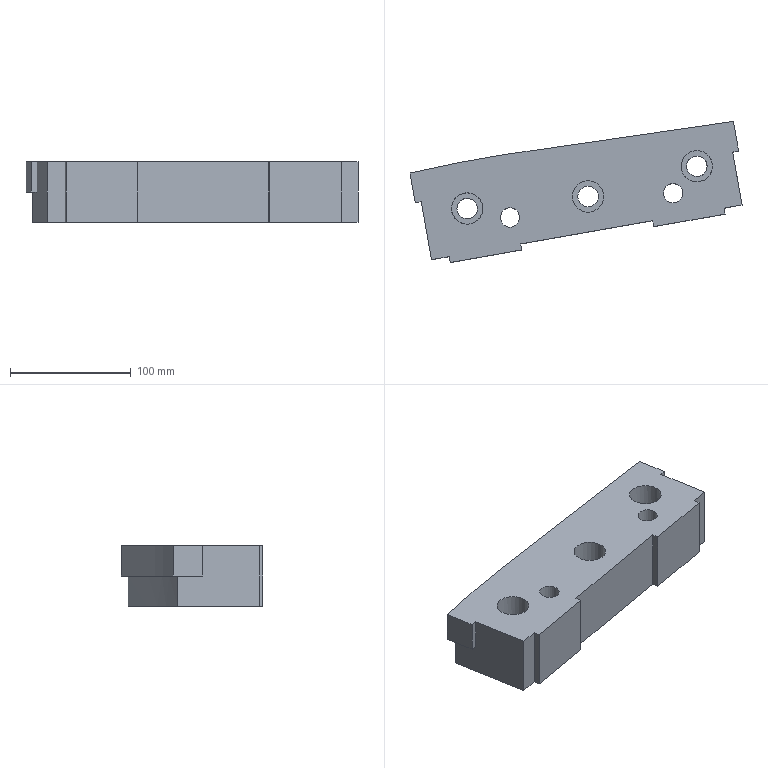Part | NX | features solid 2 | 1 solid | 31 faces | box 274.736 x 116.81 x 50 mm | volume 879881 mm3 | plane 21 | cylinder 8 | spline 2 | commonest cylinder face diameters 17 x3 26 x3 16 x2
STEP:
#1=CARTESIAN_POINT('',(-314.842,478.391,-25.));
#2=VERTEX_POINT('',#1);
#3=CARTESIAN_POINT('',(-318.361,498.353,-25.));
#4=VERTEX_POINT('',#3);
#5=CARTESIAN_POINT('',(-306.374,430.368,-25.));
#6=DIRECTION('',(0.1736,-0.9848,0.));
#7=VECTOR('',#6,1000.);
#8=LINE('',#5,#7);
#9=EDGE_CURVE('',#2,#4,#8,.F.);
#10=ORIENTED_EDGE('',*,*,#9,.F.);
#11=CARTESIAN_POINT('',(-319.766,477.523,-25.));
#12=VERTEX_POINT('',#11);
#13=CARTESIAN_POINT('',(-314.842,478.391,-25.));
#14=DIRECTION('',(-0.9848,-0.1736,0.));
#15=VECTOR('',#14,1000.);
#16=LINE('',#13,#15);
#17=EDGE_CURVE('',#2,#12,#16,.T.);
#18=ORIENTED_EDGE('',*,*,#17,.T.);
#19=CARTESIAN_POINT('',(-324.107,502.143,-25.));
#20=VERTEX_POINT('',#19);
#21=CARTESIAN_POINT('',(-314.512,447.729,-25.));
#22=DIRECTION('',(0.1736,-0.9848,0.));
#23=VECTOR('',#22,1000.);
#24=LINE('',#21,#23);
#25=EDGE_CURVE('',#20,#12,#24,.T.);
#26=ORIENTED_EDGE('',*,*,#25,.F.);
#27=CARTESIAN_POINT('',(-56.491,544.858,-25.));
#28=VERTEX_POINT('',#27);
#29=CARTESIAN_POINT('',(-56.491,544.858,-25.));
#30=CARTESIAN_POINT('',(-66.964,543.32,-25.));
#31=CARTESIAN_POINT('',(-96.659,538.867,-25.));
#32=CARTESIAN_POINT('',(-145.572,531.452,-25.));
#33=CARTESIAN_POINT('',(-203.407,523.885,-25.));
#34=CARTESIAN_POINT('',(-261.096,515.298,-25.));
#35=CARTESIAN_POINT('',(-301.27,507.478,-25.));
#36=CARTESIAN_POINT('',(-322.157,502.605,-25.));
#37=CARTESIAN_POINT('',(-324.107,502.143,-25.));
#38=B_SPLINE_CURVE_WITH_KNOTS('',3,(#29,#30,#31,#32,#33,#34,#35,#36,#37),.UNSPECIFIED.,.F.,.F.,(4,1,1,1,1,1,4),(0.,0.1171,0.3323,0.5475,0.7627,0.9778,1.),.UNSPECIFIED.);
#39=EDGE_CURVE('',#20,#28,#38,.F.);
#40=ORIENTED_EDGE('',*,*,#39,.T.);
#41=CARTESIAN_POINT('',(-52.15,520.238,-25.));
#42=VERTEX_POINT('',#41);
#43=CARTESIAN_POINT('',(-44.447,476.553,-25.));
#44=DIRECTION('',(0.1736,-0.9848,0.));
#45=VECTOR('',#44,1000.);
#46=LINE('',#43,#45);
#47=EDGE_CURVE('',#28,#42,#46,.T.);
#48=ORIENTED_EDGE('',*,*,#47,.T.);
#49=CARTESIAN_POINT('',(-57.074,519.37,-25.));
#50=VERTEX_POINT('',#49);
#51=CARTESIAN_POINT('',(-57.074,519.37,-25.));
#52=DIRECTION('',(0.9848,0.1736,0.));
#53=VECTOR('',#52,1000.);
#54=LINE('',#51,#53);
#55=EDGE_CURVE('',#50,#42,#54,.T.);
#56=ORIENTED_EDGE('',*,*,#55,.F.);
#57=CARTESIAN_POINT('',(-60.571,539.203,-25.));
#58=VERTEX_POINT('',#57);
#59=CARTESIAN_POINT('',(-49.371,475.684,-25.));
#60=DIRECTION('',(0.1736,-0.9848,0.));
#61=VECTOR('',#60,1000.);
#62=LINE('',#59,#61);
#63=EDGE_CURVE('',#50,#58,#62,.F.);
#64=ORIENTED_EDGE('',*,*,#63,.T.);
#65=CARTESIAN_POINT('',(-60.571,539.203,-25.));
#66=CARTESIAN_POINT('',(-82.108,536.021,-25.));
#67=CARTESIAN_POINT('',(-114.403,531.034,-25.));
#68=CARTESIAN_POINT('',(-157.629,524.877,-25.));
#69=CARTESIAN_POINT('',(-200.826,519.103,-25.));
#70=CARTESIAN_POINT('',(-254.61,511.408,-25.));
#71=CARTESIAN_POINT('',(-297.253,503.233,-25.));
#72=CARTESIAN_POINT('',(-318.361,498.353,-25.));
#73=B_SPLINE_CURVE_WITH_KNOTS('',3,(#65,#66,#67,#68,#69,#70,#71,#72),.UNSPECIFIED.,.F.,.F.,(4,1,1,1,1,4),(0.01794,0.2591,0.3796,0.5002,0.7414,0.9825),.UNSPECIFIED.);
#74=EDGE_CURVE('',#58,#4,#73,.T.);
#75=ORIENTED_EDGE('',*,*,#74,.T.);
#76=EDGE_LOOP('',(#10,#18,#26,#40,#48,#56,#64,#75));
#77=FACE_BOUND('',#76,.T.);
#78=CARTESIAN_POINT('',(-324.107,502.143,-25.));
#79=DIRECTION('',(0.,0.,-1.));
#80=DIRECTION('',(-0.9962,0.08716,0.));
#81=AXIS2_PLACEMENT_3D('',#78,#79,#80);
#82=PLANE('',#81);
#83=ADVANCED_FACE('',(#77),#82,.T.);
#84=CARTESIAN_POINT('',(-233.374,465.368,0.));
#85=VERTEX_POINT('',#84);
#86=CARTESIAN_POINT('',(-241.374,465.368,0.));
#87=DIRECTION('',(0.,0.,1.));
#88=DIRECTION('',(1.,0.,0.));
#89=AXIS2_PLACEMENT_3D('',#86,#87,#88);
#90=CIRCLE('',#89,8.);
#91=EDGE_CURVE('',#85,#85,#90,.T.);
#92=ORIENTED_EDGE('',*,*,#91,.F.);
#93=EDGE_LOOP('',(#92));
#94=FACE_BOUND('',#93,.T.);
#95=CARTESIAN_POINT('',(-98.374,485.368,0.));
#96=VERTEX_POINT('',#95);
#97=CARTESIAN_POINT('',(-106.374,485.368,0.));
#98=DIRECTION('',(0.,0.,1.));
#99=DIRECTION('',(1.,0.,0.));
#100=AXIS2_PLACEMENT_3D('',#97,#98,#99);
#101=CIRCLE('',#100,8.);
#102=EDGE_CURVE('',#96,#96,#101,.T.);
#103=ORIENTED_EDGE('',*,*,#102,.F.);
#104=EDGE_LOOP('',(#103));
#105=FACE_BOUND('',#104,.T.);
#106=CARTESIAN_POINT('',(-189.729,482.741,0.));
#107=VERTEX_POINT('',#106);
#108=CARTESIAN_POINT('',(-176.729,482.741,0.));
#109=DIRECTION('',(0.,0.,-1.));
#110=DIRECTION('',(-1.,0.,0.));
#111=AXIS2_PLACEMENT_3D('',#108,#109,#110);
#112=CIRCLE('',#111,13.);
#113=EDGE_CURVE('',#107,#107,#112,.T.);
#114=ORIENTED_EDGE('',*,*,#113,.T.);
#115=EDGE_LOOP('',(#114));
#116=FACE_BOUND('',#115,.T.);
#117=CARTESIAN_POINT('',(-99.729,507.741,0.));
#118=VERTEX_POINT('',#117);
#119=CARTESIAN_POINT('',(-86.729,507.741,0.));
#120=DIRECTION('',(0.,0.,-1.));
#121=DIRECTION('',(-1.,0.,0.));
#122=AXIS2_PLACEMENT_3D('',#119,#120,#121);
#123=CIRCLE('',#122,13.);
#124=EDGE_CURVE('',#118,#118,#123,.T.);
#125=ORIENTED_EDGE('',*,*,#124,.T.);
#126=EDGE_LOOP('',(#125));
#127=FACE_BOUND('',#126,.T.);
#128=CARTESIAN_POINT('',(-289.729,472.741,0.));
#129=VERTEX_POINT('',#128);
#130=CARTESIAN_POINT('',(-276.729,472.741,0.));
#131=DIRECTION('',(0.,0.,-1.));
#132=DIRECTION('',(-1.,0.,0.));
#133=AXIS2_PLACEMENT_3D('',#130,#131,#132);
#134=CIRCLE('',#133,13.);
#135=EDGE_CURVE('',#129,#129,#134,.T.);
#136=ORIENTED_EDGE('',*,*,#135,.T.);
#137=EDGE_LOOP('',(#136));
#138=FACE_BOUND('',#137,.T.);
#139=CARTESIAN_POINT('',(-319.766,477.523,0.));
#140=VERTEX_POINT('',#139);
#141=CARTESIAN_POINT('',(-324.107,502.143,0.));
#142=VERTEX_POINT('',#141);
#143=CARTESIAN_POINT('',(-314.512,447.729,0.));
#144=DIRECTION('',(-0.1736,0.9848,0.));
#145=VECTOR('',#144,1000.);
#146=LINE('',#143,#145);
#147=EDGE_CURVE('',#140,#142,#146,.T.);
#148=ORIENTED_EDGE('',*,*,#147,.F.);
#149=CARTESIAN_POINT('',(-314.842,478.391,0.));
#150=VERTEX_POINT('',#149);
#151=CARTESIAN_POINT('',(-314.842,478.391,0.));
#152=DIRECTION('',(-0.9848,-0.1736,0.));
#153=VECTOR('',#152,1000.);
#154=LINE('',#151,#153);
#155=EDGE_CURVE('',#150,#140,#154,.T.);
#156=ORIENTED_EDGE('',*,*,#155,.F.);
#157=CARTESIAN_POINT('',(-306.374,430.368,0.));
#158=VERTEX_POINT('',#157);
#159=CARTESIAN_POINT('',(-309.588,448.598,0.));
#160=DIRECTION('',(-0.1736,0.9848,0.));
#161=VECTOR('',#160,1000.);
#162=LINE('',#159,#161);
#163=EDGE_CURVE('',#158,#150,#162,.T.);
#164=ORIENTED_EDGE('',*,*,#163,.F.);
#165=CARTESIAN_POINT('',(-291.602,432.973,0.));
#166=VERTEX_POINT('',#165);
#167=CARTESIAN_POINT('',(-44.447,476.553,0.));
#168=DIRECTION('',(-0.9848,-0.1736,0.));
#169=VECTOR('',#168,1000.);
#170=LINE('',#167,#169);
#171=EDGE_CURVE('',#166,#158,#170,.T.);
#172=ORIENTED_EDGE('',*,*,#171,.F.);
#173=CARTESIAN_POINT('',(-290.733,428.048,0.));
#174=VERTEX_POINT('',#173);
#175=CARTESIAN_POINT('',(-291.602,432.973,0.));
#176=DIRECTION('',(0.1736,-0.9848,0.));
#177=VECTOR('',#176,1000.);
#178=LINE('',#175,#177);
#179=EDGE_CURVE('',#166,#174,#178,.T.);
#180=ORIENTED_EDGE('',*,*,#179,.T.);
#181=CARTESIAN_POINT('',(-231.645,438.467,0.));
#182=VERTEX_POINT('',#181);
#183=CARTESIAN_POINT('',(-241.493,436.731,0.));
#184=DIRECTION('',(-0.9848,-0.1736,0.));
#185=VECTOR('',#184,1000.);
#186=LINE('',#183,#185);
#187=EDGE_CURVE('',#182,#174,#186,.T.);
#188=ORIENTED_EDGE('',*,*,#187,.F.);
#189=CARTESIAN_POINT('',(-232.513,443.391,0.));
#190=VERTEX_POINT('',#189);
#191=CARTESIAN_POINT('',(-232.513,443.391,0.));
#192=DIRECTION('',(0.1736,-0.9848,0.));
#193=VECTOR('',#192,1000.);
#194=LINE('',#191,#193);
#195=EDGE_CURVE('',#190,#182,#194,.T.);
#196=ORIENTED_EDGE('',*,*,#195,.F.);
#197=CARTESIAN_POINT('',(-123.232,462.661,0.));
#198=VERTEX_POINT('',#197);
#199=CARTESIAN_POINT('',(-44.447,476.553,0.));
#200=DIRECTION('',(-0.9848,-0.1736,0.));
#201=VECTOR('',#200,1000.);
#202=LINE('',#199,#201);
#203=EDGE_CURVE('',#198,#190,#202,.T.);
#204=ORIENTED_EDGE('',*,*,#203,.F.);
#205=CARTESIAN_POINT('',(-122.363,457.737,0.));
#206=VERTEX_POINT('',#205);
#207=CARTESIAN_POINT('',(-123.232,462.661,0.));
#208=DIRECTION('',(0.1736,-0.9848,0.));
#209=VECTOR('',#208,1000.);
#210=LINE('',#207,#209);
#211=EDGE_CURVE('',#198,#206,#210,.T.);
#212=ORIENTED_EDGE('',*,*,#211,.T.);
#213=CARTESIAN_POINT('',(-63.275,468.156,0.));
#214=VERTEX_POINT('',#213);
#215=CARTESIAN_POINT('',(-48.503,470.76,0.));
#216=DIRECTION('',(-0.9848,-0.1736,0.));
#217=VECTOR('',#216,1000.);
#218=LINE('',#215,#217);
#219=EDGE_CURVE('',#214,#206,#218,.T.);
#220=ORIENTED_EDGE('',*,*,#219,.F.);
#221=CARTESIAN_POINT('',(-64.143,473.08,0.));
#222=VERTEX_POINT('',#221);
#223=CARTESIAN_POINT('',(-64.143,473.08,0.));
#224=DIRECTION('',(0.1736,-0.9848,0.));
#225=VECTOR('',#224,1000.);
#226=LINE('',#223,#225);
#227=EDGE_CURVE('',#222,#214,#226,.T.);
#228=ORIENTED_EDGE('',*,*,#227,.F.);
#229=CARTESIAN_POINT('',(-49.371,475.684,0.));
#230=VERTEX_POINT('',#229);
#231=CARTESIAN_POINT('',(-44.447,476.553,0.));
#232=DIRECTION('',(-0.9848,-0.1736,0.));
#233=VECTOR('',#232,1000.);
#234=LINE('',#231,#233);
#235=EDGE_CURVE('',#230,#222,#234,.T.);
#236=ORIENTED_EDGE('',*,*,#235,.F.);
#237=CARTESIAN_POINT('',(-57.074,519.37,0.));
#238=VERTEX_POINT('',#237);
#239=CARTESIAN_POINT('',(-49.371,475.684,0.));
#240=DIRECTION('',(-0.1736,0.9848,0.));
#241=VECTOR('',#240,1000.);
#242=LINE('',#239,#241);
#243=EDGE_CURVE('',#230,#238,#242,.T.);
#244=ORIENTED_EDGE('',*,*,#243,.T.);
#245=CARTESIAN_POINT('',(-52.15,520.238,0.));
#246=VERTEX_POINT('',#245);
#247=CARTESIAN_POINT('',(-57.074,519.37,0.));
#248=DIRECTION('',(0.9848,0.1736,0.));
#249=VECTOR('',#248,1000.);
#250=LINE('',#247,#249);
#251=EDGE_CURVE('',#238,#246,#250,.T.);
#252=ORIENTED_EDGE('',*,*,#251,.T.);
#253=CARTESIAN_POINT('',(-56.491,544.858,0.));
#254=VERTEX_POINT('',#253);
#255=CARTESIAN_POINT('',(-44.447,476.553,0.));
#256=DIRECTION('',(-0.1736,0.9848,0.));
#257=VECTOR('',#256,1000.);
#258=LINE('',#255,#257);
#259=EDGE_CURVE('',#246,#254,#258,.T.);
#260=ORIENTED_EDGE('',*,*,#259,.T.);
#261=CARTESIAN_POINT('',(-56.491,544.858,0.));
#262=CARTESIAN_POINT('',(-66.964,543.32,0.));
#263=CARTESIAN_POINT('',(-96.659,538.867,0.));
#264=CARTESIAN_POINT('',(-145.572,531.452,0.));
#265=CARTESIAN_POINT('',(-203.407,523.885,0.));
#266=CARTESIAN_POINT('',(-261.096,515.298,0.));
#267=CARTESIAN_POINT('',(-301.27,507.478,0.));
#268=CARTESIAN_POINT('',(-322.157,502.605,0.));
#269=CARTESIAN_POINT('',(-324.107,502.143,0.));
#270=B_SPLINE_CURVE_WITH_KNOTS('',3,(#261,#262,#263,#264,#265,#266,#267,#268,#269),.UNSPECIFIED.,.F.,.F.,(4,1,1,1,1,1,4),(0.,0.1171,0.3323,0.5475,0.7627,0.9778,1.),.UNSPECIFIED.);
#271=EDGE_CURVE('',#254,#142,#270,.T.);
#272=ORIENTED_EDGE('',*,*,#271,.T.);
#273=EDGE_LOOP('',(#148,#156,#164,#172,#180,#188,#196,#204,#212,#220,#228,#236,#244,#252,#260,#272));
#274=FACE_BOUND('',#273,.T.);
#275=CARTESIAN_POINT('',(-174.531,-853.331,0.));
#276=DIRECTION('',(0.,0.,1.));
#277=DIRECTION('',(0.9962,-0.08716,0.));
#278=AXIS2_PLACEMENT_3D('',#275,#276,#277);
#279=PLANE('',#278);
#280=ADVANCED_FACE('',(#94,#105,#116,#127,#138,#274),#279,.T.);
#281=CARTESIAN_POINT('',(-319.766,477.523,-50.));
#282=DIRECTION('',(0.,0.,-1.));
#283=VECTOR('',#282,1000.);
#284=LINE('',#281,#283);
#285=EDGE_CURVE('',#140,#12,#284,.T.);
#286=ORIENTED_EDGE('',*,*,#285,.F.);
#287=ORIENTED_EDGE('',*,*,#147,.T.);
#288=CARTESIAN_POINT('',(-324.107,502.143,-70.));
#289=DIRECTION('',(0.,0.,1.));
#290=VECTOR('',#289,1000.);
#291=LINE('',#288,#290);
#292=EDGE_CURVE('',#20,#142,#291,.T.);
#293=ORIENTED_EDGE('',*,*,#292,.F.);
#294=ORIENTED_EDGE('',*,*,#25,.T.);
#295=EDGE_LOOP('',(#286,#287,#293,#294));
#296=FACE_BOUND('',#295,.T.);
#297=CARTESIAN_POINT('',(-314.512,447.729,-50.));
#298=DIRECTION('',(0.9848,0.1736,0.));
#299=DIRECTION('',(-0.1736,0.9848,0.));
#300=AXIS2_PLACEMENT_3D('',#297,#298,#299);
#301=PLANE('',#300);
#302=ADVANCED_FACE('',(#296),#301,.F.);
#303=CARTESIAN_POINT('',(-49.371,475.684,-50.));
#304=VERTEX_POINT('',#303);
#305=CARTESIAN_POINT('',(-49.371,475.684,-50.));
#306=DIRECTION('',(0.,0.,1.));
#307=VECTOR('',#306,1000.);
#308=LINE('',#305,#307);
#309=EDGE_CURVE('',#304,#230,#308,.T.);
#310=ORIENTED_EDGE('',*,*,#309,.T.);
#311=ORIENTED_EDGE('',*,*,#235,.T.);
#312=CARTESIAN_POINT('',(-64.143,473.08,-50.));
#313=VERTEX_POINT('',#312);
#314=CARTESIAN_POINT('',(-64.143,473.08,-50.));
#315=DIRECTION('',(0.,0.,1.));
#316=VECTOR('',#315,1000.);
#317=LINE('',#314,#316);
#318=EDGE_CURVE('',#313,#222,#317,.T.);
#319=ORIENTED_EDGE('',*,*,#318,.F.);
#320=CARTESIAN_POINT('',(-44.447,476.553,-50.));
#321=DIRECTION('',(-0.9848,-0.1736,0.));
#322=VECTOR('',#321,1000.);
#323=LINE('',#320,#322);
#324=EDGE_CURVE('',#304,#313,#323,.T.);
#325=ORIENTED_EDGE('',*,*,#324,.F.);
#326=EDGE_LOOP('',(#310,#311,#319,#325));
#327=FACE_BOUND('',#326,.T.);
#328=CARTESIAN_POINT('',(-44.447,476.553,-50.));
#329=DIRECTION('',(-0.1736,0.9848,0.));
#330=DIRECTION('',(-0.9848,-0.1736,0.));
#331=AXIS2_PLACEMENT_3D('',#328,#329,#330);
#332=PLANE('',#331);
#333=ADVANCED_FACE('',(#327),#332,.F.);
#334=ORIENTED_EDGE('',*,*,#171,.T.);
#335=CARTESIAN_POINT('',(-306.374,430.368,-50.));
#336=VERTEX_POINT('',#335);
#337=CARTESIAN_POINT('',(-306.374,430.368,-50.));
#338=DIRECTION('',(0.,0.,1.));
#339=VECTOR('',#338,1000.);
#340=LINE('',#337,#339);
#341=EDGE_CURVE('',#336,#158,#340,.T.);
#342=ORIENTED_EDGE('',*,*,#341,.F.);
#343=CARTESIAN_POINT('',(-291.602,432.973,-50.));
#344=VERTEX_POINT('',#343);
#345=CARTESIAN_POINT('',(-44.447,476.553,-50.));
#346=DIRECTION('',(-0.9848,-0.1736,0.));
#347=VECTOR('',#346,1000.);
#348=LINE('',#345,#347);
#349=EDGE_CURVE('',#344,#336,#348,.T.);
#350=ORIENTED_EDGE('',*,*,#349,.F.);
#351=CARTESIAN_POINT('',(-291.602,432.973,-50.));
#352=DIRECTION('',(0.,0.,1.));
#353=VECTOR('',#352,1000.);
#354=LINE('',#351,#353);
#355=EDGE_CURVE('',#344,#166,#354,.T.);
#356=ORIENTED_EDGE('',*,*,#355,.T.);
#357=EDGE_LOOP('',(#334,#342,#350,#356));
#358=FACE_BOUND('',#357,.T.);
#359=CARTESIAN_POINT('',(-44.447,476.553,-50.));
#360=DIRECTION('',(-0.1736,0.9848,0.));
#361=DIRECTION('',(-0.9848,-0.1736,0.));
#362=AXIS2_PLACEMENT_3D('',#359,#360,#361);
#363=PLANE('',#362);
#364=ADVANCED_FACE('',(#358),#363,.F.);
#365=ORIENTED_EDGE('',*,*,#203,.T.);
#366=CARTESIAN_POINT('',(-232.513,443.391,-50.));
#367=VERTEX_POINT('',#366);
#368=CARTESIAN_POINT('',(-232.513,443.391,-50.));
#369=DIRECTION('',(0.,0.,1.));
#370=VECTOR('',#369,1000.);
#371=LINE('',#368,#370);
#372=EDGE_CURVE('',#367,#190,#371,.T.);
#373=ORIENTED_EDGE('',*,*,#372,.F.);
#374=CARTESIAN_POINT('',(-123.232,462.661,-50.));
#375=VERTEX_POINT('',#374);
#376=CARTESIAN_POINT('',(-44.447,476.553,-50.));
#377=DIRECTION('',(-0.9848,-0.1736,0.));
#378=VECTOR('',#377,1000.);
#379=LINE('',#376,#378);
#380=EDGE_CURVE('',#375,#367,#379,.T.);
#381=ORIENTED_EDGE('',*,*,#380,.F.);
#382=CARTESIAN_POINT('',(-123.232,462.661,-50.));
#383=DIRECTION('',(0.,0.,1.));
#384=VECTOR('',#383,1000.);
#385=LINE('',#382,#384);
#386=EDGE_CURVE('',#375,#198,#385,.T.);
#387=ORIENTED_EDGE('',*,*,#386,.T.);
#388=EDGE_LOOP('',(#365,#373,#381,#387));
#389=FACE_BOUND('',#388,.T.);
#390=CARTESIAN_POINT('',(-44.447,476.553,-50.));
#391=DIRECTION('',(-0.1736,0.9848,0.));
#392=DIRECTION('',(-0.9848,-0.1736,0.));
#393=AXIS2_PLACEMENT_3D('',#390,#391,#392);
#394=PLANE('',#393);
#395=ADVANCED_FACE('',(#389),#394,.F.);
#396=CARTESIAN_POINT('',(-52.15,520.238,-50.));
#397=DIRECTION('',(0.,0.,1.));
#398=VECTOR('',#397,1000.);
#399=LINE('',#396,#398);
#400=EDGE_CURVE('',#42,#246,#399,.T.);
#401=ORIENTED_EDGE('',*,*,#400,.F.);
#402=ORIENTED_EDGE('',*,*,#47,.F.);
#403=CARTESIAN_POINT('',(-56.491,544.858,-50.));
#404=DIRECTION('',(0.,0.,1.));
#405=VECTOR('',#404,1000.);
#406=LINE('',#403,#405);
#407=EDGE_CURVE('',#28,#254,#406,.T.);
#408=ORIENTED_EDGE('',*,*,#407,.T.);
#409=ORIENTED_EDGE('',*,*,#259,.F.);
#410=EDGE_LOOP('',(#401,#402,#408,#409));
#411=FACE_BOUND('',#410,.T.);
#412=CARTESIAN_POINT('',(-44.447,476.553,-50.));
#413=DIRECTION('',(0.9848,0.1736,0.));
#414=DIRECTION('',(-0.1736,0.9848,0.));
#415=AXIS2_PLACEMENT_3D('',#412,#413,#414);
#416=PLANE('',#415);
#417=ADVANCED_FACE('',(#411),#416,.T.);
#418=ORIENTED_EDGE('',*,*,#63,.F.);
#419=CARTESIAN_POINT('',(-57.074,519.37,-50.));
#420=DIRECTION('',(0.,0.,1.));
#421=VECTOR('',#420,1000.);
#422=LINE('',#419,#421);
#423=EDGE_CURVE('',#50,#238,#422,.T.);
#424=ORIENTED_EDGE('',*,*,#423,.T.);
#425=ORIENTED_EDGE('',*,*,#243,.F.);
#426=ORIENTED_EDGE('',*,*,#309,.F.);
#427=CARTESIAN_POINT('',(-60.571,539.203,-50.));
#428=VERTEX_POINT('',#427);
#429=CARTESIAN_POINT('',(-62.146,548.132,-50.));
#430=DIRECTION('',(-0.1736,0.9848,0.));
#431=VECTOR('',#430,1000.);
#432=LINE('',#429,#431);
#433=EDGE_CURVE('',#304,#428,#432,.T.);
#434=ORIENTED_EDGE('',*,*,#433,.T.);
#435=CARTESIAN_POINT('',(-60.571,539.203,-37.5));
#436=DIRECTION('',(0.,0.,-1.));
#437=VECTOR('',#436,1000.);
#438=LINE('',#435,#437);
#439=EDGE_CURVE('',#58,#428,#438,.T.);
#440=ORIENTED_EDGE('',*,*,#439,.F.);
#441=EDGE_LOOP('',(#418,#424,#425,#426,#434,#440));
#442=FACE_BOUND('',#441,.T.);
#443=CARTESIAN_POINT('',(-49.371,475.684,-25.));
#444=DIRECTION('',(-0.9848,-0.1736,0.));
#445=DIRECTION('',(0.1736,-0.9848,0.));
#446=AXIS2_PLACEMENT_3D('',#443,#444,#445);
#447=PLANE('',#446);
#448=ADVANCED_FACE('',(#442),#447,.F.);
#449=CARTESIAN_POINT('',(-122.363,457.737,-50.));
#450=VERTEX_POINT('',#449);
#451=CARTESIAN_POINT('',(-122.363,457.737,-50.));
#452=DIRECTION('',(0.,0.,1.));
#453=VECTOR('',#452,1000.);
#454=LINE('',#451,#453);
#455=EDGE_CURVE('',#450,#206,#454,.T.);
#456=ORIENTED_EDGE('',*,*,#455,.T.);
#457=ORIENTED_EDGE('',*,*,#211,.F.);
#458=ORIENTED_EDGE('',*,*,#386,.F.);
#459=CARTESIAN_POINT('',(-123.232,462.661,-50.));
#460=DIRECTION('',(0.1736,-0.9848,0.));
#461=VECTOR('',#460,1000.);
#462=LINE('',#459,#461);
#463=EDGE_CURVE('',#375,#450,#462,.T.);
#464=ORIENTED_EDGE('',*,*,#463,.T.);
#465=EDGE_LOOP('',(#456,#457,#458,#464));
#466=FACE_BOUND('',#465,.T.);
#467=CARTESIAN_POINT('',(-123.232,462.661,-50.));
#468=DIRECTION('',(0.9848,0.1736,0.));
#469=DIRECTION('',(-0.1736,0.9848,0.));
#470=AXIS2_PLACEMENT_3D('',#467,#468,#469);
#471=PLANE('',#470);
#472=ADVANCED_FACE('',(#466),#471,.F.);
#473=CARTESIAN_POINT('',(-63.275,468.156,-50.));
#474=VERTEX_POINT('',#473);
#475=CARTESIAN_POINT('',(-63.275,468.156,-50.));
#476=DIRECTION('',(0.,0.,1.));
#477=VECTOR('',#476,1000.);
#478=LINE('',#475,#477);
#479=EDGE_CURVE('',#474,#214,#478,.T.);
#480=ORIENTED_EDGE('',*,*,#479,.F.);
#481=CARTESIAN_POINT('',(-64.143,473.08,-50.));
#482=DIRECTION('',(0.1736,-0.9848,0.));
#483=VECTOR('',#482,1000.);
#484=LINE('',#481,#483);
#485=EDGE_CURVE('',#313,#474,#484,.T.);
#486=ORIENTED_EDGE('',*,*,#485,.F.);
#487=ORIENTED_EDGE('',*,*,#318,.T.);
#488=ORIENTED_EDGE('',*,*,#227,.T.);
#489=EDGE_LOOP('',(#480,#486,#487,#488));
#490=FACE_BOUND('',#489,.T.);
#491=CARTESIAN_POINT('',(-64.143,473.08,-50.));
#492=DIRECTION('',(0.9848,0.1736,0.));
#493=DIRECTION('',(-0.1736,0.9848,0.));
#494=AXIS2_PLACEMENT_3D('',#491,#492,#493);
#495=PLANE('',#494);
#496=ADVANCED_FACE('',(#490),#495,.T.);
#497=ORIENTED_EDGE('',*,*,#219,.T.);
#498=ORIENTED_EDGE('',*,*,#455,.F.);
#499=CARTESIAN_POINT('',(-48.503,470.76,-50.));
#500=DIRECTION('',(-0.9848,-0.1736,0.));
#501=VECTOR('',#500,1000.);
#502=LINE('',#499,#501);
#503=EDGE_CURVE('',#474,#450,#502,.T.);
#504=ORIENTED_EDGE('',*,*,#503,.F.);
#505=ORIENTED_EDGE('',*,*,#479,.T.);
#506=EDGE_LOOP('',(#497,#498,#504,#505));
#507=FACE_BOUND('',#506,.T.);
#508=CARTESIAN_POINT('',(-48.503,470.76,-50.));
#509=DIRECTION('',(-0.1736,0.9848,0.));
#510=DIRECTION('',(-0.9848,-0.1736,0.));
#511=AXIS2_PLACEMENT_3D('',#508,#509,#510);
#512=PLANE('',#511);
#513=ADVANCED_FACE('',(#507),#512,.F.);
#514=CARTESIAN_POINT('',(-290.733,428.048,-50.));
#515=VERTEX_POINT('',#514);
#516=CARTESIAN_POINT('',(-290.733,428.048,-50.));
#517=DIRECTION('',(0.,0.,1.));
#518=VECTOR('',#517,1000.);
#519=LINE('',#516,#518);
#520=EDGE_CURVE('',#515,#174,#519,.T.);
#521=ORIENTED_EDGE('',*,*,#520,.T.);
#522=ORIENTED_EDGE('',*,*,#179,.F.);
#523=ORIENTED_EDGE('',*,*,#355,.F.);
#524=CARTESIAN_POINT('',(-291.602,432.973,-50.));
#525=DIRECTION('',(0.1736,-0.9848,0.));
#526=VECTOR('',#525,1000.);
#527=LINE('',#524,#526);
#528=EDGE_CURVE('',#344,#515,#527,.T.);
#529=ORIENTED_EDGE('',*,*,#528,.T.);
#530=EDGE_LOOP('',(#521,#522,#523,#529));
#531=FACE_BOUND('',#530,.T.);
#532=CARTESIAN_POINT('',(-291.602,432.973,-50.));
#533=DIRECTION('',(0.9848,0.1736,0.));
#534=DIRECTION('',(-0.1736,0.9848,0.));
#535=AXIS2_PLACEMENT_3D('',#532,#533,#534);
#536=PLANE('',#535);
#537=ADVANCED_FACE('',(#531),#536,.F.);
#538=CARTESIAN_POINT('',(-231.645,438.467,-50.));
#539=VERTEX_POINT('',#538);
#540=CARTESIAN_POINT('',(-231.645,438.467,-50.));
#541=DIRECTION('',(0.,0.,1.));
#542=VECTOR('',#541,1000.);
#543=LINE('',#540,#542);
#544=EDGE_CURVE('',#539,#182,#543,.T.);
#545=ORIENTED_EDGE('',*,*,#544,.F.);
#546=CARTESIAN_POINT('',(-232.513,443.391,-50.));
#547=DIRECTION('',(0.1736,-0.9848,0.));
#548=VECTOR('',#547,1000.);
#549=LINE('',#546,#548);
#550=EDGE_CURVE('',#367,#539,#549,.T.);
#551=ORIENTED_EDGE('',*,*,#550,.F.);
#552=ORIENTED_EDGE('',*,*,#372,.T.);
#553=ORIENTED_EDGE('',*,*,#195,.T.);
#554=EDGE_LOOP('',(#545,#551,#552,#553));
#555=FACE_BOUND('',#554,.T.);
#556=CARTESIAN_POINT('',(-232.513,443.391,-50.));
#557=DIRECTION('',(0.9848,0.1736,0.));
#558=DIRECTION('',(-0.1736,0.9848,0.));
#559=AXIS2_PLACEMENT_3D('',#556,#557,#558);
#560=PLANE('',#559);
#561=ADVANCED_FACE('',(#555),#560,.T.);
#562=ORIENTED_EDGE('',*,*,#187,.T.);
#563=ORIENTED_EDGE('',*,*,#520,.F.);
#564=CARTESIAN_POINT('',(-241.493,436.731,-50.));
#565=DIRECTION('',(-0.9848,-0.1736,0.));
#566=VECTOR('',#565,1000.);
#567=LINE('',#564,#566);
#568=EDGE_CURVE('',#539,#515,#567,.T.);
#569=ORIENTED_EDGE('',*,*,#568,.F.);
#570=ORIENTED_EDGE('',*,*,#544,.T.);
#571=EDGE_LOOP('',(#562,#563,#569,#570));
#572=FACE_BOUND('',#571,.T.);
#573=CARTESIAN_POINT('',(-241.493,436.731,-50.));
#574=DIRECTION('',(-0.1736,0.9848,0.));
#575=DIRECTION('',(-0.9848,-0.1736,0.));
#576=AXIS2_PLACEMENT_3D('',#573,#574,#575);
#577=PLANE('',#576);
#578=ADVANCED_FACE('',(#572),#577,.F.);
#579=CARTESIAN_POINT('',(-233.374,465.368,-50.));
#580=VERTEX_POINT('',#579);
#581=CARTESIAN_POINT('',(-241.374,465.368,-50.));
#582=DIRECTION('',(0.,0.,1.));
#583=DIRECTION('',(1.,0.,0.));
#584=AXIS2_PLACEMENT_3D('',#581,#582,#583);
#585=CIRCLE('',#584,8.);
#586=EDGE_CURVE('',#580,#580,#585,.T.);
#587=ORIENTED_EDGE('',*,*,#586,.T.);
#588=EDGE_LOOP('',(#587));
#589=FACE_BOUND('',#588,.T.);
#590=CARTESIAN_POINT('',(-98.374,485.368,-50.));
#591=VERTEX_POINT('',#590);
#592=CARTESIAN_POINT('',(-106.374,485.368,-50.));
#593=DIRECTION('',(0.,0.,1.));
#594=DIRECTION('',(1.,0.,0.));
#595=AXIS2_PLACEMENT_3D('',#592,#593,#594);
#596=CIRCLE('',#595,8.);
#597=EDGE_CURVE('',#591,#591,#596,.T.);
#598=ORIENTED_EDGE('',*,*,#597,.T.);
#599=EDGE_LOOP('',(#598));
#600=FACE_BOUND('',#599,.T.);
#601=CARTESIAN_POINT('',(-318.361,498.353,-50.));
#602=VERTEX_POINT('',#601);
#603=CARTESIAN_POINT('',(-318.361,498.353,-50.));
#604=CARTESIAN_POINT('',(-313.473,499.483,-50.));
#605=CARTESIAN_POINT('',(-303.473,501.703,-50.));
#606=CARTESIAN_POINT('',(-290.414,504.375,-50.));
#607=CARTESIAN_POINT('',(-279.632,506.451,-50.));
#608=CARTESIAN_POINT('',(-272.754,507.723,-50.));
#609=CARTESIAN_POINT('',(-267.168,508.725,-50.));
#610=CARTESIAN_POINT('',(-262.934,509.469,-50.));
#611=CARTESIAN_POINT('',(-259.379,510.082,-50.));
#612=CARTESIAN_POINT('',(-256.857,510.51,-50.));
#613=CARTESIAN_POINT('',(-255.434,510.749,-50.));
#614=CARTESIAN_POINT('',(-254.296,510.94,-50.));
#615=CARTESIAN_POINT('',(-253.418,511.087,-50.));
#616=CARTESIAN_POINT('',(-252.148,511.297,-50.));
#617=CARTESIAN_POINT('',(-249.953,511.66,-50.));
#618=CARTESIAN_POINT('',(-245.465,512.391,-50.));
#619=CARTESIAN_POINT('',(-240.197,513.229,-50.));
#620=CARTESIAN_POINT('',(-234.775,514.071,-50.));
#621=CARTESIAN_POINT('',(-230.63,514.706,-50.));
#622=CARTESIAN_POINT('',(-227.125,515.234,-50.));
#623=CARTESIAN_POINT('',(-224.615,515.608,-50.));
#624=CARTESIAN_POINT('',(-223.208,515.817,-50.));
#625=CARTESIAN_POINT('',(-222.045,515.988,-50.));
#626=CARTESIAN_POINT('',(-221.27,516.102,-50.));
#627=CARTESIAN_POINT('',(-220.085,516.276,-50.));
#628=CARTESIAN_POINT('',(-218.042,516.575,-50.));
#629=CARTESIAN_POINT('',(-214.992,517.017,-50.));
#630=CARTESIAN_POINT('',(-211.19,517.562,-50.));
#631=CARTESIAN_POINT('',(-205.908,518.312,-50.));
#632=CARTESIAN_POINT('',(-200.311,519.096,-50.));
#633=CARTESIAN_POINT('',(-195.15,519.809,-50.));
#634=CARTESIAN_POINT('',(-192.486,520.176,-50.));
#635=CARTESIAN_POINT('',(-190.969,520.384,-50.));
#636=CARTESIAN_POINT('',(-189.751,520.551,-50.));
#637=CARTESIAN_POINT('',(-188.795,520.681,-50.));
#638=CARTESIAN_POINT('',(-187.43,520.868,-50.));
#639=CARTESIAN_POINT('',(-185.083,521.189,-50.));
#640=CARTESIAN_POINT('',(-180.359,521.834,-50.));
#641=CARTESIAN_POINT('',(-174.972,522.568,-50.));
#642=CARTESIAN_POINT('',(-169.581,523.302,-50.));
#643=CARTESIAN_POINT('',(-165.536,523.852,-50.));
#644=CARTESIAN_POINT('',(-162.175,524.308,-50.));
#645=CARTESIAN_POINT('',(-159.803,524.63,-50.));
#646=CARTESIAN_POINT('',(-158.477,524.81,-50.));
#647=CARTESIAN_POINT('',(-157.398,524.956,-50.));
#648=CARTESIAN_POINT('',(-156.642,525.059,-50.));
#649=CARTESIAN_POINT('',(-155.501,525.215,-50.));
#650=CARTESIAN_POINT('',(-153.517,525.487,-50.));
#651=CARTESIAN_POINT('',(-149.345,526.064,-50.));
#652=CARTESIAN_POINT('',(-144.216,526.787,-50.));
#653=CARTESIAN_POINT('',(-138.704,527.575,-50.));
#654=CARTESIAN_POINT('',(-135.101,528.095,-50.));
#655=CARTESIAN_POINT('',(-132.126,528.527,-50.));
#656=CARTESIAN_POINT('',(-129.843,528.859,-50.));
#657=CARTESIAN_POINT('',(-127.914,529.141,-50.));
#658=CARTESIAN_POINT('',(-126.518,529.346,-50.));
#659=CARTESIAN_POINT('',(-125.755,529.458,-50.));
#660=CARTESIAN_POINT('',(-125.063,529.56,-50.));
#661=CARTESIAN_POINT('',(-124.814,529.596,-50.));
#662=CARTESIAN_POINT('',(-124.318,529.669,-50.));
#663=CARTESIAN_POINT('',(-123.506,529.789,-50.));
#664=CARTESIAN_POINT('',(-122.256,529.973,-50.));
#665=CARTESIAN_POINT('',(-120.691,530.205,-50.));
#666=CARTESIAN_POINT('',(-118.49,530.531,-50.));
#667=CARTESIAN_POINT('',(-115.536,530.97,-50.));
#668=CARTESIAN_POINT('',(-110.375,531.74,-50.));
#669=CARTESIAN_POINT('',(-104.548,532.613,-50.));
#670=CARTESIAN_POINT('',(-98.102,533.582,-50.));
#671=CARTESIAN_POINT('',(-92.849,534.372,-50.));
#672=CARTESIAN_POINT('',(-87.62,535.16,-50.));
#673=CARTESIAN_POINT('',(-81.184,536.127,-50.));
#674=CARTESIAN_POINT('',(-73.909,537.218,-50.));
#675=CARTESIAN_POINT('',(-66.488,538.326,-50.));
#676=CARTESIAN_POINT('',(-62.4,538.933,-50.));
#677=CARTESIAN_POINT('',(-60.571,539.203,-50.));
#678=B_SPLINE_CURVE_WITH_KNOTS('',3,(#603,#604,#605,#606,#607,#608,#609,#610,#611,#612,#613,#614,#615,#616,#617,#618,#619,#620,#621,#622,#623,#624,#625,#626,#627,#628,#629,#630,#631,#632,#633,#634,#635,#636,#637,#638,#639,#640,#641,#642,#643,#644,#645,#646,#647,#648,#649,#650,#651,#652,#653,#654,#655,#656,#657,#658,#659,#660,#661,#662,#663,#664,#665,#666,#667,#668,#669,#670,#671,#672,#673,#674,#675,#676,#677),.UNSPECIFIED.,.F.,.F.,(4,1,1,1,1,1,1,1,1,1,1,1,1,1,1,1,1,1,1,1,1,1,1,1,1,1,1,1,1,1,1,1,1,1,1,1,1,1,1,1,1,1,1,1,1,1,1,1,1,1,1,1,1,1,1,1,1,1,1,1,1,1,1,1,1,1,1,1,1,1,1,1,4),(0.,0.0625,0.125,0.1562,0.1875,0.2031,0.2188,0.2344,0.2422,0.2461,0.25,0.2539,0.2578,0.2656,0.2812,0.3125,0.3281,0.3438,0.3594,0.3672,0.3711,0.375,0.3789,0.3828,0.3906,0.4062,0.4219,0.4375,0.4688,0.4844,0.4922,0.4961,0.5,0.5039,0.5078,0.5156,0.5312,0.5625,0.5781,0.5938,0.6094,0.6172,0.6211,0.625,0.6289,0.6328,0.6406,0.6562,0.6875,0.7031,0.7188,0.7266,0.7344,0.7422,0.7461,0.748,0.75,0.752,0.7539,0.7578,0.7656,0.7734,0.7812,0.7969,0.8125,0.8438,0.8594,0.875,0.8906,0.9062,0.9375,0.9688,1.),.UNSPECIFIED.);
#679=EDGE_CURVE('',#428,#602,#678,.F.);
#680=ORIENTED_EDGE('',*,*,#679,.F.);
#681=ORIENTED_EDGE('',*,*,#433,.F.);
#682=ORIENTED_EDGE('',*,*,#324,.T.);
#683=ORIENTED_EDGE('',*,*,#485,.T.);
#684=ORIENTED_EDGE('',*,*,#503,.T.);
#685=ORIENTED_EDGE('',*,*,#463,.F.);
#686=ORIENTED_EDGE('',*,*,#380,.T.);
#687=ORIENTED_EDGE('',*,*,#550,.T.);
#688=ORIENTED_EDGE('',*,*,#568,.T.);
#689=ORIENTED_EDGE('',*,*,#528,.F.);
#690=ORIENTED_EDGE('',*,*,#349,.T.);
#691=CARTESIAN_POINT('',(-319.148,502.816,-50.));
#692=DIRECTION('',(-0.1736,0.9848,0.));
#693=VECTOR('',#692,1000.);
#694=LINE('',#691,#693);
#695=EDGE_CURVE('',#336,#602,#694,.T.);
#696=ORIENTED_EDGE('',*,*,#695,.T.);
#697=EDGE_LOOP('',(#680,#681,#682,#683,#684,#685,#686,#687,#688,#689,#690,#696));
#698=FACE_BOUND('',#697,.T.);
#699=CARTESIAN_POINT('',(-285.229,472.741,-50.));
#700=VERTEX_POINT('',#699);
#701=CARTESIAN_POINT('',(-276.729,472.741,-50.));
#702=DIRECTION('',(0.,0.,-1.));
#703=DIRECTION('',(-1.,0.,0.));
#704=AXIS2_PLACEMENT_3D('',#701,#702,#703);
#705=CIRCLE('',#704,8.5);
#706=EDGE_CURVE('',#700,#700,#705,.T.);
#707=ORIENTED_EDGE('',*,*,#706,.F.);
#708=EDGE_LOOP('',(#707));
#709=FACE_BOUND('',#708,.T.);
#710=CARTESIAN_POINT('',(-95.229,507.741,-50.));
#711=VERTEX_POINT('',#710);
#712=CARTESIAN_POINT('',(-86.729,507.741,-50.));
#713=DIRECTION('',(0.,0.,-1.));
#714=DIRECTION('',(-1.,0.,0.));
#715=AXIS2_PLACEMENT_3D('',#712,#713,#714);
#716=CIRCLE('',#715,8.5);
#717=EDGE_CURVE('',#711,#711,#716,.T.);
#718=ORIENTED_EDGE('',*,*,#717,.F.);
#719=EDGE_LOOP('',(#718));
#720=FACE_BOUND('',#719,.T.);
#721=CARTESIAN_POINT('',(-185.229,482.741,-50.));
#722=VERTEX_POINT('',#721);
#723=CARTESIAN_POINT('',(-176.729,482.741,-50.));
#724=DIRECTION('',(0.,0.,-1.));
#725=DIRECTION('',(-1.,0.,0.));
#726=AXIS2_PLACEMENT_3D('',#723,#724,#725);
#727=CIRCLE('',#726,8.5);
#728=EDGE_CURVE('',#722,#722,#727,.T.);
#729=ORIENTED_EDGE('',*,*,#728,.F.);
#730=EDGE_LOOP('',(#729));
#731=FACE_BOUND('',#730,.T.);
#732=CARTESIAN_POINT('',(-174.531,-853.331,-50.));
#733=DIRECTION('',(0.,0.,1.));
#734=DIRECTION('',(0.9962,-0.08716,0.));
#735=AXIS2_PLACEMENT_3D('',#732,#733,#734);
#736=PLANE('',#735);
#737=ADVANCED_FACE('',(#589,#600,#698,#709,#720,#731),#736,.F.);
#738=CARTESIAN_POINT('',(-276.729,481.241,-25.));
#739=VERTEX_POINT('',#738);
#740=CARTESIAN_POINT('',(-276.729,472.741,-25.));
#741=DIRECTION('',(0.,0.,-1.));
#742=DIRECTION('',(0.,1.,0.));
#743=AXIS2_PLACEMENT_3D('',#740,#741,#742);
#744=CIRCLE('',#743,8.5);
#745=EDGE_CURVE('',#739,#739,#744,.F.);
#746=ORIENTED_EDGE('',*,*,#745,.F.);
#747=EDGE_LOOP('',(#746));
#748=FACE_BOUND('',#747,.T.);
#749=CARTESIAN_POINT('',(-276.729,459.741,-25.));
#750=VERTEX_POINT('',#749);
#751=CARTESIAN_POINT('',(-276.729,472.741,-25.));
#752=DIRECTION('',(0.,0.,1.));
#753=DIRECTION('',(0.,-1.,0.));
#754=AXIS2_PLACEMENT_3D('',#751,#752,#753);
#755=CIRCLE('',#754,13.);
#756=EDGE_CURVE('',#750,#750,#755,.T.);
#757=ORIENTED_EDGE('',*,*,#756,.T.);
#758=EDGE_LOOP('',(#757));
#759=FACE_BOUND('',#758,.T.);
#760=CARTESIAN_POINT('',(-276.729,472.741,-25.));
#761=DIRECTION('',(0.,0.,-1.));
#762=DIRECTION('',(0.,1.,0.));
#763=AXIS2_PLACEMENT_3D('',#760,#761,#762);
#764=PLANE('',#763);
#765=ADVANCED_FACE('',(#748,#759),#764,.F.);
#766=ORIENTED_EDGE('',*,*,#706,.T.);
#767=EDGE_LOOP('',(#766));
#768=FACE_BOUND('',#767,.T.);
#769=ORIENTED_EDGE('',*,*,#745,.T.);
#770=EDGE_LOOP('',(#769));
#771=FACE_BOUND('',#770,.T.);
#772=CARTESIAN_POINT('',(-276.729,472.741,-75.));
#773=DIRECTION('',(0.,0.,1.));
#774=DIRECTION('',(0.,-1.,0.));
#775=AXIS2_PLACEMENT_3D('',#772,#773,#774);
#776=CYLINDRICAL_SURFACE('',#775,8.5);
#777=ADVANCED_FACE('',(#768,#771),#776,.F.);
#778=ORIENTED_EDGE('',*,*,#135,.F.);
#779=EDGE_LOOP('',(#778));
#780=FACE_BOUND('',#779,.T.);
#781=ORIENTED_EDGE('',*,*,#756,.F.);
#782=EDGE_LOOP('',(#781));
#783=FACE_BOUND('',#782,.T.);
#784=CARTESIAN_POINT('',(-276.729,472.741,-25.));
#785=DIRECTION('',(0.,0.,1.));
#786=DIRECTION('',(0.,-1.,0.));
#787=AXIS2_PLACEMENT_3D('',#784,#785,#786);
#788=CYLINDRICAL_SURFACE('',#787,13.);
#789=ADVANCED_FACE('',(#780,#783),#788,.F.);
#790=CARTESIAN_POINT('',(-163.729,482.741,-25.));
#791=VERTEX_POINT('',#790);
#792=CARTESIAN_POINT('',(-176.729,482.741,-25.));
#793=DIRECTION('',(0.,0.,1.));
#794=DIRECTION('',(1.,0.,0.));
#795=AXIS2_PLACEMENT_3D('',#792,#793,#794);
#796=CIRCLE('',#795,13.);
#797=EDGE_CURVE('',#791,#791,#796,.T.);
#798=ORIENTED_EDGE('',*,*,#797,.T.);
#799=EDGE_LOOP('',(#798));
#800=FACE_BOUND('',#799,.T.);
#801=CARTESIAN_POINT('',(-185.229,482.741,-25.));
#802=VERTEX_POINT('',#801);
#803=CARTESIAN_POINT('',(-176.729,482.741,-25.));
#804=DIRECTION('',(0.,0.,-1.));
#805=DIRECTION('',(-1.,0.,0.));
#806=AXIS2_PLACEMENT_3D('',#803,#804,#805);
#807=CIRCLE('',#806,8.5);
#808=EDGE_CURVE('',#802,#802,#807,.F.);
#809=ORIENTED_EDGE('',*,*,#808,.F.);
#810=EDGE_LOOP('',(#809));
#811=FACE_BOUND('',#810,.T.);
#812=CARTESIAN_POINT('',(-176.729,482.741,-25.));
#813=DIRECTION('',(0.,0.,-1.));
#814=DIRECTION('',(-1.,0.,0.));
#815=AXIS2_PLACEMENT_3D('',#812,#813,#814);
#816=PLANE('',#815);
#817=ADVANCED_FACE('',(#800,#811),#816,.F.);
#818=ORIENTED_EDGE('',*,*,#113,.F.);
#819=EDGE_LOOP('',(#818));
#820=FACE_BOUND('',#819,.T.);
#821=ORIENTED_EDGE('',*,*,#797,.F.);
#822=EDGE_LOOP('',(#821));
#823=FACE_BOUND('',#822,.T.);
#824=CARTESIAN_POINT('',(-176.729,482.741,-25.));
#825=DIRECTION('',(0.,0.,1.));
#826=DIRECTION('',(1.,0.,0.));
#827=AXIS2_PLACEMENT_3D('',#824,#825,#826);
#828=CYLINDRICAL_SURFACE('',#827,13.);
#829=ADVANCED_FACE('',(#820,#823),#828,.F.);
#830=ORIENTED_EDGE('',*,*,#728,.T.);
#831=EDGE_LOOP('',(#830));
#832=FACE_BOUND('',#831,.T.);
#833=ORIENTED_EDGE('',*,*,#808,.T.);
#834=EDGE_LOOP('',(#833));
#835=FACE_BOUND('',#834,.T.);
#836=CARTESIAN_POINT('',(-176.729,482.741,-75.));
#837=DIRECTION('',(0.,0.,1.));
#838=DIRECTION('',(1.,0.,0.));
#839=AXIS2_PLACEMENT_3D('',#836,#837,#838);
#840=CYLINDRICAL_SURFACE('',#839,8.5);
#841=ADVANCED_FACE('',(#832,#835),#840,.F.);
#842=CARTESIAN_POINT('',(-86.729,516.241,-25.));
#843=VERTEX_POINT('',#842);
#844=CARTESIAN_POINT('',(-86.729,507.741,-25.));
#845=DIRECTION('',(0.,0.,-1.));
#846=DIRECTION('',(0.,1.,0.));
#847=AXIS2_PLACEMENT_3D('',#844,#845,#846);
#848=CIRCLE('',#847,8.5);
#849=EDGE_CURVE('',#843,#843,#848,.F.);
#850=ORIENTED_EDGE('',*,*,#849,.F.);
#851=EDGE_LOOP('',(#850));
#852=FACE_BOUND('',#851,.T.);
#853=CARTESIAN_POINT('',(-86.729,494.741,-25.));
#854=VERTEX_POINT('',#853);
#855=CARTESIAN_POINT('',(-86.729,507.741,-25.));
#856=DIRECTION('',(0.,0.,1.));
#857=DIRECTION('',(0.,-1.,0.));
#858=AXIS2_PLACEMENT_3D('',#855,#856,#857);
#859=CIRCLE('',#858,13.);
#860=EDGE_CURVE('',#854,#854,#859,.T.);
#861=ORIENTED_EDGE('',*,*,#860,.T.);
#862=EDGE_LOOP('',(#861));
#863=FACE_BOUND('',#862,.T.);
#864=CARTESIAN_POINT('',(-86.729,507.741,-25.));
#865=DIRECTION('',(0.,0.,-1.));
#866=DIRECTION('',(0.,1.,0.));
#867=AXIS2_PLACEMENT_3D('',#864,#865,#866);
#868=PLANE('',#867);
#869=ADVANCED_FACE('',(#852,#863),#868,.F.);
#870=ORIENTED_EDGE('',*,*,#717,.T.);
#871=EDGE_LOOP('',(#870));
#872=FACE_BOUND('',#871,.T.);
#873=ORIENTED_EDGE('',*,*,#849,.T.);
#874=EDGE_LOOP('',(#873));
#875=FACE_BOUND('',#874,.T.);
#876=CARTESIAN_POINT('',(-86.729,507.741,-75.));
#877=DIRECTION('',(0.,0.,1.));
#878=DIRECTION('',(0.,-1.,0.));
#879=AXIS2_PLACEMENT_3D('',#876,#877,#878);
#880=CYLINDRICAL_SURFACE('',#879,8.5);
#881=ADVANCED_FACE('',(#872,#875),#880,.F.);
#882=ORIENTED_EDGE('',*,*,#124,.F.);
#883=EDGE_LOOP('',(#882));
#884=FACE_BOUND('',#883,.T.);
#885=ORIENTED_EDGE('',*,*,#860,.F.);
#886=EDGE_LOOP('',(#885));
#887=FACE_BOUND('',#886,.T.);
#888=CARTESIAN_POINT('',(-86.729,507.741,-25.));
#889=DIRECTION('',(0.,0.,1.));
#890=DIRECTION('',(0.,-1.,0.));
#891=AXIS2_PLACEMENT_3D('',#888,#889,#890);
#892=CYLINDRICAL_SURFACE('',#891,13.);
#893=ADVANCED_FACE('',(#884,#887),#892,.F.);
#894=ORIENTED_EDGE('',*,*,#39,.F.);
#895=ORIENTED_EDGE('',*,*,#292,.T.);
#896=ORIENTED_EDGE('',*,*,#271,.F.);
#897=ORIENTED_EDGE('',*,*,#407,.F.);
#898=EDGE_LOOP('',(#894,#895,#896,#897));
#899=FACE_BOUND('',#898,.T.);
#900=CARTESIAN_POINT('',(-56.491,544.858,-25.));
#901=CARTESIAN_POINT('',(-56.491,544.858,0.));
#902=CARTESIAN_POINT('',(-78.841,541.576,-25.));
#903=CARTESIAN_POINT('',(-78.841,541.576,0.));
#904=CARTESIAN_POINT('',(-112.329,536.401,-25.));
#905=CARTESIAN_POINT('',(-112.329,536.401,0.));
#906=CARTESIAN_POINT('',(-157.051,529.998,-25.));
#907=CARTESIAN_POINT('',(-157.051,529.998,0.));
#908=CARTESIAN_POINT('',(-201.832,524.017,-25.));
#909=CARTESIAN_POINT('',(-201.832,524.017,0.));
#910=CARTESIAN_POINT('',(-257.73,516.008,-25.));
#911=CARTESIAN_POINT('',(-257.73,516.008,0.));
#912=CARTESIAN_POINT('',(-302.125,507.355,-25.));
#913=CARTESIAN_POINT('',(-302.125,507.355,0.));
#914=CARTESIAN_POINT('',(-324.107,502.143,-25.));
#915=CARTESIAN_POINT('',(-324.107,502.143,0.));
#916=B_SPLINE_SURFACE_WITH_KNOTS('',3,1,((#900,#901),(#902,#903),(#904,#905),(#906,#907),(#908,#909),(#910,#911),(#912,#913),(#914,#915)),.SURF_OF_LINEAR_EXTRUSION.,.F.,.F.,.F.,(4,1,1,1,1,4),(2,2),(0.,0.25,0.375,0.5,0.75,1.),(0.,1.),.UNSPECIFIED.);
#917=ADVANCED_FACE('',(#899),#916,.T.);
#918=ORIENTED_EDGE('',*,*,#695,.F.);
#919=ORIENTED_EDGE('',*,*,#341,.T.);
#920=ORIENTED_EDGE('',*,*,#163,.T.);
#921=CARTESIAN_POINT('',(-314.842,478.391,-70.));
#922=DIRECTION('',(0.,0.,1.));
#923=VECTOR('',#922,1000.);
#924=LINE('',#921,#923);
#925=EDGE_CURVE('',#2,#150,#924,.T.);
#926=ORIENTED_EDGE('',*,*,#925,.F.);
#927=ORIENTED_EDGE('',*,*,#9,.T.);
#928=CARTESIAN_POINT('',(-318.361,498.353,-37.5));
#929=DIRECTION('',(0.,0.,-1.));
#930=VECTOR('',#929,1000.);
#931=LINE('',#928,#930);
#932=EDGE_CURVE('',#4,#602,#931,.T.);
#933=ORIENTED_EDGE('',*,*,#932,.T.);
#934=EDGE_LOOP('',(#918,#919,#920,#926,#927,#933));
#935=FACE_BOUND('',#934,.T.);
#936=CARTESIAN_POINT('',(-306.374,430.368,-25.));
#937=DIRECTION('',(-0.9848,-0.1736,0.));
#938=DIRECTION('',(0.1736,-0.9848,0.));
#939=AXIS2_PLACEMENT_3D('',#936,#937,#938);
#940=PLANE('',#939);
#941=ADVANCED_FACE('',(#935),#940,.T.);
#942=ORIENTED_EDGE('',*,*,#74,.F.);
#943=ORIENTED_EDGE('',*,*,#439,.T.);
#944=ORIENTED_EDGE('',*,*,#679,.T.);
#945=ORIENTED_EDGE('',*,*,#932,.F.);
#946=EDGE_LOOP('',(#942,#943,#944,#945));
#947=FACE_BOUND('',#946,.T.);
#948=CARTESIAN_POINT('',(-60.571,539.203,-25.));
#949=CARTESIAN_POINT('',(-60.571,539.203,-50.));
#950=CARTESIAN_POINT('',(-82.108,536.021,-25.));
#951=CARTESIAN_POINT('',(-82.108,536.021,-50.));
#952=CARTESIAN_POINT('',(-114.403,531.034,-25.));
#953=CARTESIAN_POINT('',(-114.403,531.034,-50.));
#954=CARTESIAN_POINT('',(-157.629,524.877,-25.));
#955=CARTESIAN_POINT('',(-157.629,524.877,-50.));
#956=CARTESIAN_POINT('',(-200.826,519.103,-25.));
#957=CARTESIAN_POINT('',(-200.826,519.103,-50.));
#958=CARTESIAN_POINT('',(-254.61,511.408,-25.));
#959=CARTESIAN_POINT('',(-254.61,511.408,-50.));
#960=CARTESIAN_POINT('',(-297.253,503.233,-25.));
#961=CARTESIAN_POINT('',(-297.253,503.233,-50.));
#962=CARTESIAN_POINT('',(-318.361,498.353,-25.));
#963=CARTESIAN_POINT('',(-318.361,498.353,-50.));
#964=B_SPLINE_SURFACE_WITH_KNOTS('',3,1,((#948,#949),(#950,#951),(#952,#953),(#954,#955),(#956,#957),(#958,#959),(#960,#961),(#962,#963)),.SURF_OF_LINEAR_EXTRUSION.,.F.,.F.,.F.,(4,1,1,1,1,4),(2,2),(0.01794,0.2591,0.3796,0.5002,0.7414,0.9825),(0.,1.),.UNSPECIFIED.);
#965=ADVANCED_FACE('',(#947),#964,.F.);
#966=ORIENTED_EDGE('',*,*,#400,.T.);
#967=ORIENTED_EDGE('',*,*,#251,.F.);
#968=ORIENTED_EDGE('',*,*,#423,.F.);
#969=ORIENTED_EDGE('',*,*,#55,.T.);
#970=EDGE_LOOP('',(#966,#967,#968,#969));
#971=FACE_BOUND('',#970,.T.);
#972=CARTESIAN_POINT('',(-57.074,519.37,-50.));
#973=DIRECTION('',(-0.1736,0.9848,0.));
#974=DIRECTION('',(-0.9848,-0.1736,0.));
#975=AXIS2_PLACEMENT_3D('',#972,#973,#974);
#976=PLANE('',#975);
#977=ADVANCED_FACE('',(#971),#976,.F.);
#978=ORIENTED_EDGE('',*,*,#285,.T.);
#979=ORIENTED_EDGE('',*,*,#17,.F.);
#980=ORIENTED_EDGE('',*,*,#925,.T.);
#981=ORIENTED_EDGE('',*,*,#155,.T.);
#982=EDGE_LOOP('',(#978,#979,#980,#981));
#983=FACE_BOUND('',#982,.T.);
#984=CARTESIAN_POINT('',(-314.842,478.391,-70.));
#985=DIRECTION('',(0.1736,-0.9848,0.));
#986=DIRECTION('',(0.9848,0.1736,0.));
#987=AXIS2_PLACEMENT_3D('',#984,#985,#986);
#988=PLANE('',#987);
#989=ADVANCED_FACE('',(#983),#988,.T.);
#990=ORIENTED_EDGE('',*,*,#102,.T.);
#991=EDGE_LOOP('',(#990));
#992=FACE_BOUND('',#991,.T.);
#993=ORIENTED_EDGE('',*,*,#597,.F.);
#994=EDGE_LOOP('',(#993));
#995=FACE_BOUND('',#994,.T.);
#996=CARTESIAN_POINT('',(-106.374,485.368,50.));
#997=DIRECTION('',(0.,0.,-1.));
#998=DIRECTION('',(-1.,0.,0.));
#999=AXIS2_PLACEMENT_3D('',#996,#997,#998);
#1000=CYLINDRICAL_SURFACE('',#999,8.);
#1001=ADVANCED_FACE('',(#992,#995),#1000,.F.);
#1002=ORIENTED_EDGE('',*,*,#91,.T.);
#1003=EDGE_LOOP('',(#1002));
#1004=FACE_BOUND('',#1003,.T.);
#1005=ORIENTED_EDGE('',*,*,#586,.F.);
#1006=EDGE_LOOP('',(#1005));
#1007=FACE_BOUND('',#1006,.T.);
#1008=CARTESIAN_POINT('',(-241.374,465.368,50.));
#1009=DIRECTION('',(0.,0.,-1.));
#1010=DIRECTION('',(-1.,0.,0.));
#1011=AXIS2_PLACEMENT_3D('',#1008,#1009,#1010);
#1012=CYLINDRICAL_SURFACE('',#1011,8.);
#1013=ADVANCED_FACE('',(#1004,#1007),#1012,.F.);
#1014=CLOSED_SHELL('',(#83,#280,#302,#333,#364,#395,#417,#448,#472,#496,#513,#537,#561,#578,#737,#765,#777,#789,#817,#829,#841,#869,#881,#893,#917,#941,#965,#977,#989,#1001,#1013));
#1015=MANIFOLD_SOLID_BREP('',#1014);
#1016=(LENGTH_UNIT()NAMED_UNIT(*)SI_UNIT(.MILLI.,.METRE.));
#1017=UNCERTAINTY_MEASURE_WITH_UNIT(LENGTH_MEASURE(0.0508),#1016,'','');
#1018=(NAMED_UNIT(*)PLANE_ANGLE_UNIT()SI_UNIT($,.RADIAN.));
#1019=(NAMED_UNIT(*)SI_UNIT($,.STERADIAN.)SOLID_ANGLE_UNIT());
#1020=(GEOMETRIC_REPRESENTATION_CONTEXT(3)GLOBAL_UNCERTAINTY_ASSIGNED_CONTEXT((#1017))GLOBAL_UNIT_ASSIGNED_CONTEXT((#1016,#1018,#1019))REPRESENTATION_CONTEXT('',''));
#1021=ADVANCED_BREP_SHAPE_REPRESENTATION('',(#1015),#1020);